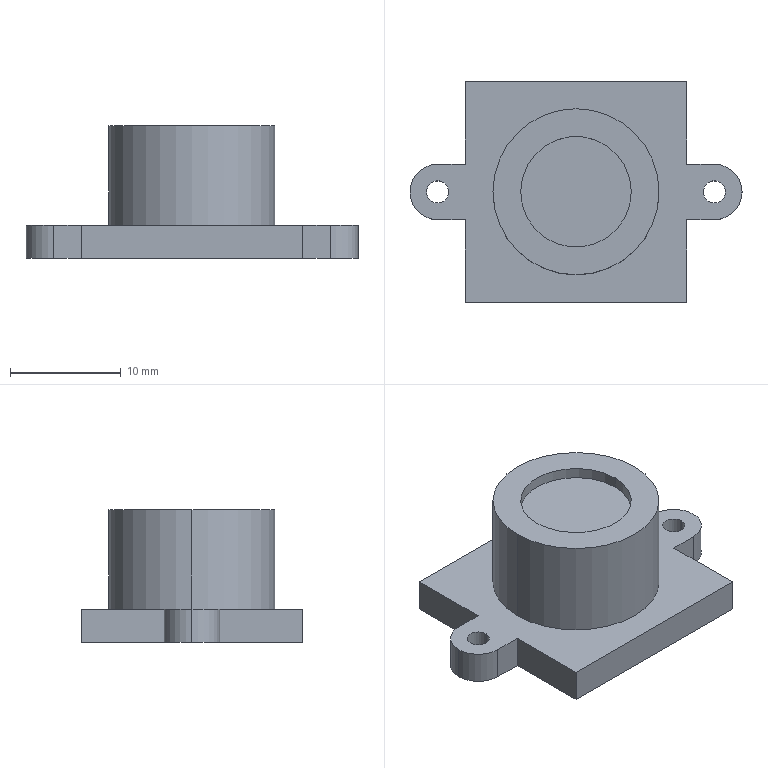Part | SolidWorks | features ICE 4, Extrusion 1, Fillet 1, MirrorPattern 1 | 1 solid | 26 faces | box 30 x 20 x 12 mm | volume 2827 mm3 | plane 14 | cylinder 12 | commonest cylinder face diameters 2 x4 5 x4 10 x2 15 x2
STEP:
#1=CARTESIAN_POINT('',(-5.,0.,11.));
#2=VERTEX_POINT('',#1);
#3=CARTESIAN_POINT('',(5.,0.,11.));
#4=VERTEX_POINT('',#3);
#5=CARTESIAN_POINT('',(0.,0.,11.));
#6=DIRECTION('',(0.,0.,1.));
#7=DIRECTION('',(1.,0.,0.));
#8=AXIS2_PLACEMENT_3D('',#5,#6,#7);
#9=CIRCLE('',#8,5.);
#10=EDGE_CURVE('',#2,#4,#9,.T.);
#11=ORIENTED_EDGE('',*,*,#10,.F.);
#12=CARTESIAN_POINT('',(-5.,0.,12.));
#13=VERTEX_POINT('',#12);
#14=CARTESIAN_POINT('',(-5.,0.,11.));
#15=DIRECTION('',(0.,0.,1.));
#16=VECTOR('',#15,1000.);
#17=LINE('',#14,#16);
#18=EDGE_CURVE('',#2,#13,#17,.T.);
#19=ORIENTED_EDGE('',*,*,#18,.T.);
#20=CARTESIAN_POINT('',(5.,0.,12.));
#21=VERTEX_POINT('',#20);
#22=CARTESIAN_POINT('',(0.,0.,12.));
#23=DIRECTION('',(0.,0.,1.));
#24=DIRECTION('',(1.,0.,0.));
#25=AXIS2_PLACEMENT_3D('',#22,#23,#24);
#26=CIRCLE('',#25,5.);
#27=EDGE_CURVE('',#13,#21,#26,.T.);
#28=ORIENTED_EDGE('',*,*,#27,.T.);
#29=CARTESIAN_POINT('',(5.,0.,11.));
#30=DIRECTION('',(0.,0.,1.));
#31=VECTOR('',#30,1000.);
#32=LINE('',#29,#31);
#33=EDGE_CURVE('',#4,#21,#32,.T.);
#34=ORIENTED_EDGE('',*,*,#33,.F.);
#35=EDGE_LOOP('',(#11,#19,#28,#34));
#36=FACE_OUTER_BOUND('',#35,.T.);
#37=CARTESIAN_POINT('',(0.,0.,11.));
#38=DIRECTION('',(0.,0.,1.));
#39=DIRECTION('',(1.,0.,0.));
#40=AXIS2_PLACEMENT_3D('',#37,#38,#39);
#41=CYLINDRICAL_SURFACE('',#40,5.);
#42=ADVANCED_FACE('',(#36),#41,.F.);
#43=CARTESIAN_POINT('',(7.5,0.,12.));
#44=VERTEX_POINT('',#43);
#45=CARTESIAN_POINT('',(-7.5,0.,12.));
#46=VERTEX_POINT('',#45);
#47=CARTESIAN_POINT('',(0.,0.,12.));
#48=DIRECTION('',(0.,0.,1.));
#49=DIRECTION('',(1.,0.,0.));
#50=AXIS2_PLACEMENT_3D('',#47,#48,#49);
#51=CIRCLE('',#50,7.5);
#52=EDGE_CURVE('',#44,#46,#51,.T.);
#53=ORIENTED_EDGE('',*,*,#52,.F.);
#54=CARTESIAN_POINT('',(7.5,0.,3.));
#55=VERTEX_POINT('',#54);
#56=CARTESIAN_POINT('',(7.5,0.,12.));
#57=DIRECTION('',(0.,0.,-1.));
#58=VECTOR('',#57,1000.);
#59=LINE('',#56,#58);
#60=EDGE_CURVE('',#44,#55,#59,.T.);
#61=ORIENTED_EDGE('',*,*,#60,.T.);
#62=CARTESIAN_POINT('',(-7.5,0.,3.));
#63=VERTEX_POINT('',#62);
#64=CARTESIAN_POINT('',(0.,0.,3.));
#65=DIRECTION('',(0.,0.,1.));
#66=DIRECTION('',(1.,0.,0.));
#67=AXIS2_PLACEMENT_3D('',#64,#65,#66);
#68=CIRCLE('',#67,7.5);
#69=EDGE_CURVE('',#55,#63,#68,.T.);
#70=ORIENTED_EDGE('',*,*,#69,.T.);
#71=CARTESIAN_POINT('',(-7.5,0.,12.));
#72=DIRECTION('',(0.,0.,-1.));
#73=VECTOR('',#72,1000.);
#74=LINE('',#71,#73);
#75=EDGE_CURVE('',#46,#63,#74,.T.);
#76=ORIENTED_EDGE('',*,*,#75,.F.);
#77=EDGE_LOOP('',(#53,#61,#70,#76));
#78=FACE_OUTER_BOUND('',#77,.T.);
#79=CARTESIAN_POINT('',(0.,0.,12.));
#80=DIRECTION('',(0.,0.,-1.));
#81=DIRECTION('',(-1.,0.,0.));
#82=AXIS2_PLACEMENT_3D('',#79,#80,#81);
#83=CYLINDRICAL_SURFACE('',#82,7.5);
#84=ADVANCED_FACE('',(#78),#83,.T.);
#85=CARTESIAN_POINT('',(11.5,0.,0.));
#86=VERTEX_POINT('',#85);
#87=CARTESIAN_POINT('',(13.5,0.,0.));
#88=VERTEX_POINT('',#87);
#89=CARTESIAN_POINT('',(12.5,0.,0.));
#90=DIRECTION('',(0.,0.,1.));
#91=DIRECTION('',(1.,0.,0.));
#92=AXIS2_PLACEMENT_3D('',#89,#90,#91);
#93=CIRCLE('',#92,1.);
#94=EDGE_CURVE('',#86,#88,#93,.T.);
#95=ORIENTED_EDGE('',*,*,#94,.F.);
#96=CARTESIAN_POINT('',(11.5,0.,3.));
#97=VERTEX_POINT('',#96);
#98=CARTESIAN_POINT('',(11.5,0.,-2.828));
#99=DIRECTION('',(0.,0.,1.));
#100=VECTOR('',#99,1000.);
#101=LINE('',#98,#100);
#102=EDGE_CURVE('',#86,#97,#101,.T.);
#103=ORIENTED_EDGE('',*,*,#102,.T.);
#104=CARTESIAN_POINT('',(13.5,0.,3.));
#105=VERTEX_POINT('',#104);
#106=CARTESIAN_POINT('',(12.5,0.,3.));
#107=DIRECTION('',(0.,0.,-1.));
#108=DIRECTION('',(-1.,0.,0.));
#109=AXIS2_PLACEMENT_3D('',#106,#107,#108);
#110=CIRCLE('',#109,1.);
#111=EDGE_CURVE('',#105,#97,#110,.T.);
#112=ORIENTED_EDGE('',*,*,#111,.F.);
#113=CARTESIAN_POINT('',(13.5,0.,-2.828));
#114=DIRECTION('',(0.,0.,1.));
#115=VECTOR('',#114,1000.);
#116=LINE('',#113,#115);
#117=EDGE_CURVE('',#88,#105,#116,.T.);
#118=ORIENTED_EDGE('',*,*,#117,.F.);
#119=EDGE_LOOP('',(#95,#103,#112,#118));
#120=FACE_OUTER_BOUND('',#119,.T.);
#121=CARTESIAN_POINT('',(12.5,0.,-2.828));
#122=DIRECTION('',(0.,0.,1.));
#123=DIRECTION('',(1.,0.,0.));
#124=AXIS2_PLACEMENT_3D('',#121,#122,#123);
#125=CYLINDRICAL_SURFACE('',#124,1.);
#126=ADVANCED_FACE('',(#120),#125,.F.);
#127=CARTESIAN_POINT('',(-11.5,0.,0.));
#128=VERTEX_POINT('',#127);
#129=CARTESIAN_POINT('',(-13.5,0.,0.));
#130=VERTEX_POINT('',#129);
#131=CARTESIAN_POINT('',(-12.5,0.,0.));
#132=DIRECTION('',(0.,0.,-1.));
#133=DIRECTION('',(1.,0.,0.));
#134=AXIS2_PLACEMENT_3D('',#131,#132,#133);
#135=CIRCLE('',#134,1.);
#136=EDGE_CURVE('',#128,#130,#135,.T.);
#137=ORIENTED_EDGE('',*,*,#136,.T.);
#138=CARTESIAN_POINT('',(-13.5,0.,3.));
#139=VERTEX_POINT('',#138);
#140=CARTESIAN_POINT('',(-13.5,0.,-2.828));
#141=DIRECTION('',(0.,0.,1.));
#142=VECTOR('',#141,1000.);
#143=LINE('',#140,#142);
#144=EDGE_CURVE('',#130,#139,#143,.T.);
#145=ORIENTED_EDGE('',*,*,#144,.T.);
#146=CARTESIAN_POINT('',(-11.5,0.,3.));
#147=VERTEX_POINT('',#146);
#148=CARTESIAN_POINT('',(-12.5,0.,3.));
#149=DIRECTION('',(0.,0.,1.));
#150=DIRECTION('',(1.,0.,0.));
#151=AXIS2_PLACEMENT_3D('',#148,#149,#150);
#152=CIRCLE('',#151,1.);
#153=EDGE_CURVE('',#139,#147,#152,.T.);
#154=ORIENTED_EDGE('',*,*,#153,.T.);
#155=CARTESIAN_POINT('',(-11.5,0.,-2.828));
#156=DIRECTION('',(0.,0.,1.));
#157=VECTOR('',#156,1000.);
#158=LINE('',#155,#157);
#159=EDGE_CURVE('',#128,#147,#158,.T.);
#160=ORIENTED_EDGE('',*,*,#159,.F.);
#161=EDGE_LOOP('',(#137,#145,#154,#160));
#162=FACE_OUTER_BOUND('',#161,.T.);
#163=CARTESIAN_POINT('',(-12.5,0.,-2.828));
#164=DIRECTION('',(0.,0.,1.));
#165=DIRECTION('',(1.,0.,0.));
#166=AXIS2_PLACEMENT_3D('',#163,#164,#165);
#167=CYLINDRICAL_SURFACE('',#166,1.);
#168=ADVANCED_FACE('',(#162),#167,.F.);
#169=CARTESIAN_POINT('',(10.,2.5,0.));
#170=VERTEX_POINT('',#169);
#171=CARTESIAN_POINT('',(10.,2.5,3.));
#172=VERTEX_POINT('',#171);
#173=CARTESIAN_POINT('',(10.,2.5,-7.071));
#174=DIRECTION('',(0.,0.,1.));
#175=VECTOR('',#174,1000.);
#176=LINE('',#173,#175);
#177=EDGE_CURVE('',#170,#172,#176,.T.);
#178=ORIENTED_EDGE('',*,*,#177,.F.);
#179=CARTESIAN_POINT('',(10.,10.,0.));
#180=VERTEX_POINT('',#179);
#181=CARTESIAN_POINT('',(10.,10.,0.));
#182=DIRECTION('',(0.,1.,0.));
#183=VECTOR('',#182,1000.);
#184=LINE('',#181,#183);
#185=EDGE_CURVE('',#170,#180,#184,.T.);
#186=ORIENTED_EDGE('',*,*,#185,.T.);
#187=CARTESIAN_POINT('',(10.,10.,3.));
#188=VERTEX_POINT('',#187);
#189=CARTESIAN_POINT('',(10.,10.,3.));
#190=DIRECTION('',(0.,0.,-1.));
#191=VECTOR('',#190,1000.);
#192=LINE('',#189,#191);
#193=EDGE_CURVE('',#188,#180,#192,.T.);
#194=ORIENTED_EDGE('',*,*,#193,.F.);
#195=CARTESIAN_POINT('',(10.,10.,3.));
#196=DIRECTION('',(0.,1.,0.));
#197=VECTOR('',#196,1000.);
#198=LINE('',#195,#197);
#199=EDGE_CURVE('',#172,#188,#198,.T.);
#200=ORIENTED_EDGE('',*,*,#199,.F.);
#201=EDGE_LOOP('',(#178,#186,#194,#200));
#202=FACE_OUTER_BOUND('',#201,.T.);
#203=CARTESIAN_POINT('',(10.,10.,3.));
#204=DIRECTION('',(-1.,0.,0.));
#205=DIRECTION('',(0.,-1.,0.));
#206=AXIS2_PLACEMENT_3D('',#203,#204,#205);
#207=PLANE('',#206);
#208=ADVANCED_FACE('',(#202),#207,.F.);
#209=CARTESIAN_POINT('',(-10.,-2.5,0.));
#210=VERTEX_POINT('',#209);
#211=CARTESIAN_POINT('',(-10.,-2.5,3.));
#212=VERTEX_POINT('',#211);
#213=CARTESIAN_POINT('',(-10.,-2.5,-7.071));
#214=DIRECTION('',(0.,0.,1.));
#215=VECTOR('',#214,1000.);
#216=LINE('',#213,#215);
#217=EDGE_CURVE('',#210,#212,#216,.T.);
#218=ORIENTED_EDGE('',*,*,#217,.F.);
#219=CARTESIAN_POINT('',(-10.,-10.,0.));
#220=VERTEX_POINT('',#219);
#221=CARTESIAN_POINT('',(-10.,10.,0.));
#222=DIRECTION('',(0.,-1.,0.));
#223=VECTOR('',#222,1000.);
#224=LINE('',#221,#223);
#225=EDGE_CURVE('',#210,#220,#224,.T.);
#226=ORIENTED_EDGE('',*,*,#225,.T.);
#227=CARTESIAN_POINT('',(-10.,-10.,3.));
#228=VERTEX_POINT('',#227);
#229=CARTESIAN_POINT('',(-10.,-10.,3.));
#230=DIRECTION('',(0.,0.,-1.));
#231=VECTOR('',#230,1000.);
#232=LINE('',#229,#231);
#233=EDGE_CURVE('',#228,#220,#232,.T.);
#234=ORIENTED_EDGE('',*,*,#233,.F.);
#235=CARTESIAN_POINT('',(-10.,10.,3.));
#236=DIRECTION('',(0.,-1.,0.));
#237=VECTOR('',#236,1000.);
#238=LINE('',#235,#237);
#239=EDGE_CURVE('',#212,#228,#238,.T.);
#240=ORIENTED_EDGE('',*,*,#239,.F.);
#241=EDGE_LOOP('',(#218,#226,#234,#240));
#242=FACE_OUTER_BOUND('',#241,.T.);
#243=CARTESIAN_POINT('',(-10.,10.,3.));
#244=DIRECTION('',(1.,0.,0.));
#245=DIRECTION('',(0.,1.,0.));
#246=AXIS2_PLACEMENT_3D('',#243,#244,#245);
#247=PLANE('',#246);
#248=ADVANCED_FACE('',(#242),#247,.F.);
#249=CARTESIAN_POINT('',(10.,-10.,0.));
#250=VERTEX_POINT('',#249);
#251=CARTESIAN_POINT('',(10.,-2.5,0.));
#252=VERTEX_POINT('',#251);
#253=CARTESIAN_POINT('',(10.,10.,0.));
#254=DIRECTION('',(0.,1.,0.));
#255=VECTOR('',#254,1000.);
#256=LINE('',#253,#255);
#257=EDGE_CURVE('',#250,#252,#256,.T.);
#258=ORIENTED_EDGE('',*,*,#257,.T.);
#259=CARTESIAN_POINT('',(10.,-2.5,3.));
#260=VERTEX_POINT('',#259);
#261=CARTESIAN_POINT('',(10.,-2.5,-7.071));
#262=DIRECTION('',(0.,0.,1.));
#263=VECTOR('',#262,1000.);
#264=LINE('',#261,#263);
#265=EDGE_CURVE('',#252,#260,#264,.T.);
#266=ORIENTED_EDGE('',*,*,#265,.T.);
#267=CARTESIAN_POINT('',(10.,-10.,3.));
#268=VERTEX_POINT('',#267);
#269=CARTESIAN_POINT('',(10.,10.,3.));
#270=DIRECTION('',(0.,1.,0.));
#271=VECTOR('',#270,1000.);
#272=LINE('',#269,#271);
#273=EDGE_CURVE('',#268,#260,#272,.T.);
#274=ORIENTED_EDGE('',*,*,#273,.F.);
#275=CARTESIAN_POINT('',(10.,-10.,3.));
#276=DIRECTION('',(0.,0.,-1.));
#277=VECTOR('',#276,1000.);
#278=LINE('',#275,#277);
#279=EDGE_CURVE('',#268,#250,#278,.T.);
#280=ORIENTED_EDGE('',*,*,#279,.T.);
#281=EDGE_LOOP('',(#258,#266,#274,#280));
#282=FACE_OUTER_BOUND('',#281,.T.);
#283=CARTESIAN_POINT('',(10.,10.,3.));
#284=DIRECTION('',(-1.,0.,0.));
#285=DIRECTION('',(0.,-1.,0.));
#286=AXIS2_PLACEMENT_3D('',#283,#284,#285);
#287=PLANE('',#286);
#288=ADVANCED_FACE('',(#282),#287,.F.);
#289=CARTESIAN_POINT('',(-10.,10.,0.));
#290=VERTEX_POINT('',#289);
#291=CARTESIAN_POINT('',(-10.,10.,0.));
#292=DIRECTION('',(-1.,0.,0.));
#293=VECTOR('',#292,1000.);
#294=LINE('',#291,#293);
#295=EDGE_CURVE('',#180,#290,#294,.T.);
#296=ORIENTED_EDGE('',*,*,#295,.T.);
#297=CARTESIAN_POINT('',(-10.,10.,3.));
#298=VERTEX_POINT('',#297);
#299=CARTESIAN_POINT('',(-10.,10.,3.));
#300=DIRECTION('',(0.,0.,-1.));
#301=VECTOR('',#300,1000.);
#302=LINE('',#299,#301);
#303=EDGE_CURVE('',#298,#290,#302,.T.);
#304=ORIENTED_EDGE('',*,*,#303,.F.);
#305=CARTESIAN_POINT('',(-10.,10.,3.));
#306=DIRECTION('',(-1.,0.,0.));
#307=VECTOR('',#306,1000.);
#308=LINE('',#305,#307);
#309=EDGE_CURVE('',#188,#298,#308,.T.);
#310=ORIENTED_EDGE('',*,*,#309,.F.);
#311=ORIENTED_EDGE('',*,*,#193,.T.);
#312=EDGE_LOOP('',(#296,#304,#310,#311));
#313=FACE_OUTER_BOUND('',#312,.T.);
#314=CARTESIAN_POINT('',(-10.,10.,3.));
#315=DIRECTION('',(0.,-1.,0.));
#316=DIRECTION('',(0.,0.,-1.));
#317=AXIS2_PLACEMENT_3D('',#314,#315,#316);
#318=PLANE('',#317);
#319=ADVANCED_FACE('',(#313),#318,.F.);
#320=CARTESIAN_POINT('',(-10.,2.5,0.));
#321=VERTEX_POINT('',#320);
#322=CARTESIAN_POINT('',(-10.,10.,0.));
#323=DIRECTION('',(0.,-1.,0.));
#324=VECTOR('',#323,1000.);
#325=LINE('',#322,#324);
#326=EDGE_CURVE('',#290,#321,#325,.T.);
#327=ORIENTED_EDGE('',*,*,#326,.T.);
#328=CARTESIAN_POINT('',(-10.,2.5,3.));
#329=VERTEX_POINT('',#328);
#330=CARTESIAN_POINT('',(-10.,2.5,-7.071));
#331=DIRECTION('',(0.,0.,1.));
#332=VECTOR('',#331,1000.);
#333=LINE('',#330,#332);
#334=EDGE_CURVE('',#321,#329,#333,.T.);
#335=ORIENTED_EDGE('',*,*,#334,.T.);
#336=CARTESIAN_POINT('',(-10.,10.,3.));
#337=DIRECTION('',(0.,-1.,0.));
#338=VECTOR('',#337,1000.);
#339=LINE('',#336,#338);
#340=EDGE_CURVE('',#298,#329,#339,.T.);
#341=ORIENTED_EDGE('',*,*,#340,.F.);
#342=ORIENTED_EDGE('',*,*,#303,.T.);
#343=EDGE_LOOP('',(#327,#335,#341,#342));
#344=FACE_OUTER_BOUND('',#343,.T.);
#345=CARTESIAN_POINT('',(-10.,10.,3.));
#346=DIRECTION('',(1.,0.,0.));
#347=DIRECTION('',(0.,1.,0.));
#348=AXIS2_PLACEMENT_3D('',#345,#346,#347);
#349=PLANE('',#348);
#350=ADVANCED_FACE('',(#344),#349,.F.);
#351=CARTESIAN_POINT('',(-10.,-10.,0.));
#352=DIRECTION('',(1.,0.,0.));
#353=VECTOR('',#352,1000.);
#354=LINE('',#351,#353);
#355=EDGE_CURVE('',#220,#250,#354,.T.);
#356=ORIENTED_EDGE('',*,*,#355,.T.);
#357=ORIENTED_EDGE('',*,*,#279,.F.);
#358=CARTESIAN_POINT('',(-10.,-10.,3.));
#359=DIRECTION('',(1.,0.,0.));
#360=VECTOR('',#359,1000.);
#361=LINE('',#358,#360);
#362=EDGE_CURVE('',#228,#268,#361,.T.);
#363=ORIENTED_EDGE('',*,*,#362,.F.);
#364=ORIENTED_EDGE('',*,*,#233,.T.);
#365=EDGE_LOOP('',(#356,#357,#363,#364));
#366=FACE_OUTER_BOUND('',#365,.T.);
#367=CARTESIAN_POINT('',(-10.,-10.,3.));
#368=DIRECTION('',(0.,1.,0.));
#369=DIRECTION('',(0.,0.,1.));
#370=AXIS2_PLACEMENT_3D('',#367,#368,#369);
#371=PLANE('',#370);
#372=ADVANCED_FACE('',(#366),#371,.F.);
#373=CARTESIAN_POINT('',(0.,0.,3.));
#374=DIRECTION('',(0.,0.,1.));
#375=DIRECTION('',(1.,0.,0.));
#376=AXIS2_PLACEMENT_3D('',#373,#374,#375);
#377=CIRCLE('',#376,7.5);
#378=EDGE_CURVE('',#63,#55,#377,.T.);
#379=ORIENTED_EDGE('',*,*,#378,.F.);
#380=ORIENTED_EDGE('',*,*,#69,.F.);
#381=EDGE_LOOP('',(#379,#380));
#382=FACE_BOUND('',#381,.T.);
#383=ORIENTED_EDGE('',*,*,#111,.T.);
#384=CARTESIAN_POINT('',(12.5,0.,3.));
#385=DIRECTION('',(0.,0.,-1.));
#386=DIRECTION('',(-1.,0.,0.));
#387=AXIS2_PLACEMENT_3D('',#384,#385,#386);
#388=CIRCLE('',#387,1.);
#389=EDGE_CURVE('',#97,#105,#388,.T.);
#390=ORIENTED_EDGE('',*,*,#389,.T.);
#391=EDGE_LOOP('',(#383,#390));
#392=FACE_BOUND('',#391,.T.);
#393=CARTESIAN_POINT('',(-12.5,0.,3.));
#394=DIRECTION('',(0.,0.,1.));
#395=DIRECTION('',(1.,0.,0.));
#396=AXIS2_PLACEMENT_3D('',#393,#394,#395);
#397=CIRCLE('',#396,1.);
#398=EDGE_CURVE('',#147,#139,#397,.T.);
#399=ORIENTED_EDGE('',*,*,#398,.F.);
#400=ORIENTED_EDGE('',*,*,#153,.F.);
#401=EDGE_LOOP('',(#399,#400));
#402=FACE_BOUND('',#401,.T.);
#403=CARTESIAN_POINT('',(12.5,-2.5,3.));
#404=VERTEX_POINT('',#403);
#405=CARTESIAN_POINT('',(15.,0.,3.));
#406=VERTEX_POINT('',#405);
#407=CARTESIAN_POINT('',(12.5,0.,3.));
#408=DIRECTION('',(0.,0.,1.));
#409=DIRECTION('',(1.,0.,0.));
#410=AXIS2_PLACEMENT_3D('',#407,#408,#409);
#411=CIRCLE('',#410,2.5);
#412=EDGE_CURVE('',#404,#406,#411,.T.);
#413=ORIENTED_EDGE('',*,*,#412,.T.);
#414=CARTESIAN_POINT('',(12.5,2.5,3.));
#415=VERTEX_POINT('',#414);
#416=CARTESIAN_POINT('',(12.5,0.,3.));
#417=DIRECTION('',(0.,0.,1.));
#418=DIRECTION('',(1.,0.,0.));
#419=AXIS2_PLACEMENT_3D('',#416,#417,#418);
#420=CIRCLE('',#419,2.5);
#421=EDGE_CURVE('',#406,#415,#420,.T.);
#422=ORIENTED_EDGE('',*,*,#421,.T.);
#423=CARTESIAN_POINT('',(10.,2.5,3.));
#424=DIRECTION('',(1.,0.,0.));
#425=VECTOR('',#424,1000.);
#426=LINE('',#423,#425);
#427=EDGE_CURVE('',#172,#415,#426,.T.);
#428=ORIENTED_EDGE('',*,*,#427,.F.);
#429=ORIENTED_EDGE('',*,*,#199,.T.);
#430=ORIENTED_EDGE('',*,*,#309,.T.);
#431=ORIENTED_EDGE('',*,*,#340,.T.);
#432=CARTESIAN_POINT('',(-12.5,2.5,3.));
#433=VERTEX_POINT('',#432);
#434=CARTESIAN_POINT('',(-10.,2.5,3.));
#435=DIRECTION('',(-1.,0.,0.));
#436=VECTOR('',#435,1000.);
#437=LINE('',#434,#436);
#438=EDGE_CURVE('',#329,#433,#437,.T.);
#439=ORIENTED_EDGE('',*,*,#438,.T.);
#440=CARTESIAN_POINT('',(-15.,0.,3.));
#441=VERTEX_POINT('',#440);
#442=CARTESIAN_POINT('',(-12.5,0.,3.));
#443=DIRECTION('',(0.,0.,1.));
#444=DIRECTION('',(1.,0.,0.));
#445=AXIS2_PLACEMENT_3D('',#442,#443,#444);
#446=CIRCLE('',#445,2.5);
#447=EDGE_CURVE('',#433,#441,#446,.T.);
#448=ORIENTED_EDGE('',*,*,#447,.T.);
#449=CARTESIAN_POINT('',(-12.5,-2.5,3.));
#450=VERTEX_POINT('',#449);
#451=CARTESIAN_POINT('',(-12.5,0.,3.));
#452=DIRECTION('',(0.,0.,1.));
#453=DIRECTION('',(1.,0.,0.));
#454=AXIS2_PLACEMENT_3D('',#451,#452,#453);
#455=CIRCLE('',#454,2.5);
#456=EDGE_CURVE('',#441,#450,#455,.T.);
#457=ORIENTED_EDGE('',*,*,#456,.T.);
#458=CARTESIAN_POINT('',(-15.,-2.5,3.));
#459=DIRECTION('',(1.,0.,0.));
#460=VECTOR('',#459,1000.);
#461=LINE('',#458,#460);
#462=EDGE_CURVE('',#450,#212,#461,.T.);
#463=ORIENTED_EDGE('',*,*,#462,.T.);
#464=ORIENTED_EDGE('',*,*,#239,.T.);
#465=ORIENTED_EDGE('',*,*,#362,.T.);
#466=ORIENTED_EDGE('',*,*,#273,.T.);
#467=CARTESIAN_POINT('',(15.,-2.5,3.));
#468=DIRECTION('',(-1.,0.,0.));
#469=VECTOR('',#468,1000.);
#470=LINE('',#467,#469);
#471=EDGE_CURVE('',#404,#260,#470,.T.);
#472=ORIENTED_EDGE('',*,*,#471,.F.);
#473=EDGE_LOOP('',(#413,#422,#428,#429,#430,#431,#439,#448,#457,#463,#464,#465,#466,#472));
#474=FACE_OUTER_BOUND('',#473,.T.);
#475=CARTESIAN_POINT('',(0.,0.,3.));
#476=DIRECTION('',(0.,0.,1.));
#477=DIRECTION('',(1.,0.,0.));
#478=AXIS2_PLACEMENT_3D('',#475,#476,#477);
#479=PLANE('',#478);
#480=ADVANCED_FACE('',(#382,#392,#402,#474),#479,.T.);
#481=CARTESIAN_POINT('',(12.5,0.,0.));
#482=DIRECTION('',(0.,0.,1.));
#483=DIRECTION('',(1.,0.,0.));
#484=AXIS2_PLACEMENT_3D('',#481,#482,#483);
#485=CIRCLE('',#484,1.);
#486=EDGE_CURVE('',#88,#86,#485,.T.);
#487=ORIENTED_EDGE('',*,*,#486,.T.);
#488=ORIENTED_EDGE('',*,*,#94,.T.);
#489=EDGE_LOOP('',(#487,#488));
#490=FACE_BOUND('',#489,.T.);
#491=ORIENTED_EDGE('',*,*,#136,.F.);
#492=CARTESIAN_POINT('',(-12.5,0.,0.));
#493=DIRECTION('',(0.,0.,-1.));
#494=DIRECTION('',(1.,0.,0.));
#495=AXIS2_PLACEMENT_3D('',#492,#493,#494);
#496=CIRCLE('',#495,1.);
#497=EDGE_CURVE('',#130,#128,#496,.T.);
#498=ORIENTED_EDGE('',*,*,#497,.F.);
#499=EDGE_LOOP('',(#491,#498));
#500=FACE_BOUND('',#499,.T.);
#501=CARTESIAN_POINT('',(12.5,2.5,0.));
#502=VERTEX_POINT('',#501);
#503=CARTESIAN_POINT('',(10.,2.5,0.));
#504=DIRECTION('',(-1.,0.,0.));
#505=VECTOR('',#504,1000.);
#506=LINE('',#503,#505);
#507=EDGE_CURVE('',#502,#170,#506,.T.);
#508=ORIENTED_EDGE('',*,*,#507,.F.);
#509=CARTESIAN_POINT('',(15.,0.,0.));
#510=VERTEX_POINT('',#509);
#511=CARTESIAN_POINT('',(12.5,0.,0.));
#512=DIRECTION('',(0.,0.,-1.));
#513=DIRECTION('',(1.,0.,0.));
#514=AXIS2_PLACEMENT_3D('',#511,#512,#513);
#515=CIRCLE('',#514,2.5);
#516=EDGE_CURVE('',#502,#510,#515,.T.);
#517=ORIENTED_EDGE('',*,*,#516,.T.);
#518=CARTESIAN_POINT('',(12.5,-2.5,0.));
#519=VERTEX_POINT('',#518);
#520=CARTESIAN_POINT('',(12.5,0.,0.));
#521=DIRECTION('',(0.,0.,-1.));
#522=DIRECTION('',(1.,0.,0.));
#523=AXIS2_PLACEMENT_3D('',#520,#521,#522);
#524=CIRCLE('',#523,2.5);
#525=EDGE_CURVE('',#510,#519,#524,.T.);
#526=ORIENTED_EDGE('',*,*,#525,.T.);
#527=CARTESIAN_POINT('',(15.,-2.5,0.));
#528=DIRECTION('',(1.,0.,0.));
#529=VECTOR('',#528,1000.);
#530=LINE('',#527,#529);
#531=EDGE_CURVE('',#252,#519,#530,.T.);
#532=ORIENTED_EDGE('',*,*,#531,.F.);
#533=ORIENTED_EDGE('',*,*,#257,.F.);
#534=ORIENTED_EDGE('',*,*,#355,.F.);
#535=ORIENTED_EDGE('',*,*,#225,.F.);
#536=CARTESIAN_POINT('',(-12.5,-2.5,0.));
#537=VERTEX_POINT('',#536);
#538=CARTESIAN_POINT('',(-15.,-2.5,0.));
#539=DIRECTION('',(-1.,0.,0.));
#540=VECTOR('',#539,1000.);
#541=LINE('',#538,#540);
#542=EDGE_CURVE('',#210,#537,#541,.T.);
#543=ORIENTED_EDGE('',*,*,#542,.T.);
#544=CARTESIAN_POINT('',(-15.,0.,0.));
#545=VERTEX_POINT('',#544);
#546=CARTESIAN_POINT('',(-12.5,0.,0.));
#547=DIRECTION('',(0.,0.,-1.));
#548=DIRECTION('',(1.,0.,0.));
#549=AXIS2_PLACEMENT_3D('',#546,#547,#548);
#550=CIRCLE('',#549,2.5);
#551=EDGE_CURVE('',#537,#545,#550,.T.);
#552=ORIENTED_EDGE('',*,*,#551,.T.);
#553=CARTESIAN_POINT('',(-12.5,2.5,0.));
#554=VERTEX_POINT('',#553);
#555=CARTESIAN_POINT('',(-12.5,0.,0.));
#556=DIRECTION('',(0.,0.,-1.));
#557=DIRECTION('',(1.,0.,0.));
#558=AXIS2_PLACEMENT_3D('',#555,#556,#557);
#559=CIRCLE('',#558,2.5);
#560=EDGE_CURVE('',#545,#554,#559,.T.);
#561=ORIENTED_EDGE('',*,*,#560,.T.);
#562=CARTESIAN_POINT('',(-10.,2.5,0.));
#563=DIRECTION('',(1.,0.,0.));
#564=VECTOR('',#563,1000.);
#565=LINE('',#562,#564);
#566=EDGE_CURVE('',#554,#321,#565,.T.);
#567=ORIENTED_EDGE('',*,*,#566,.T.);
#568=ORIENTED_EDGE('',*,*,#326,.F.);
#569=ORIENTED_EDGE('',*,*,#295,.F.);
#570=ORIENTED_EDGE('',*,*,#185,.F.);
#571=EDGE_LOOP('',(#508,#517,#526,#532,#533,#534,#535,#543,#552,#561,#567,#568,#569,#570));
#572=FACE_OUTER_BOUND('',#571,.T.);
#573=CARTESIAN_POINT('',(0.,0.,0.));
#574=DIRECTION('',(0.,0.,1.));
#575=DIRECTION('',(1.,0.,0.));
#576=AXIS2_PLACEMENT_3D('',#573,#574,#575);
#577=PLANE('',#576);
#578=ADVANCED_FACE('',(#490,#500,#572),#577,.F.);
#579=ORIENTED_EDGE('',*,*,#462,.F.);
#580=CARTESIAN_POINT('',(-12.5,-2.5,-7.071));
#581=DIRECTION('',(0.,0.,-1.));
#582=VECTOR('',#581,1000.);
#583=LINE('',#580,#582);
#584=EDGE_CURVE('',#450,#537,#583,.T.);
#585=ORIENTED_EDGE('',*,*,#584,.T.);
#586=ORIENTED_EDGE('',*,*,#542,.F.);
#587=ORIENTED_EDGE('',*,*,#217,.T.);
#588=EDGE_LOOP('',(#579,#585,#586,#587));
#589=FACE_OUTER_BOUND('',#588,.T.);
#590=CARTESIAN_POINT('',(-15.,-2.5,-7.071));
#591=DIRECTION('',(0.,-1.,0.));
#592=DIRECTION('',(1.,0.,0.));
#593=AXIS2_PLACEMENT_3D('',#590,#591,#592);
#594=PLANE('',#593);
#595=ADVANCED_FACE('',(#589),#594,.T.);
#596=ORIENTED_EDGE('',*,*,#566,.F.);
#597=CARTESIAN_POINT('',(-12.5,2.5,-7.071));
#598=DIRECTION('',(0.,0.,1.));
#599=VECTOR('',#598,1000.);
#600=LINE('',#597,#599);
#601=EDGE_CURVE('',#554,#433,#600,.T.);
#602=ORIENTED_EDGE('',*,*,#601,.T.);
#603=ORIENTED_EDGE('',*,*,#438,.F.);
#604=ORIENTED_EDGE('',*,*,#334,.F.);
#605=EDGE_LOOP('',(#596,#602,#603,#604));
#606=FACE_OUTER_BOUND('',#605,.T.);
#607=CARTESIAN_POINT('',(-10.,2.5,-7.071));
#608=DIRECTION('',(0.,1.,0.));
#609=DIRECTION('',(-1.,0.,0.));
#610=AXIS2_PLACEMENT_3D('',#607,#608,#609);
#611=PLANE('',#610);
#612=ADVANCED_FACE('',(#606),#611,.T.);
#613=ORIENTED_EDGE('',*,*,#144,.F.);
#614=ORIENTED_EDGE('',*,*,#497,.T.);
#615=ORIENTED_EDGE('',*,*,#159,.T.);
#616=ORIENTED_EDGE('',*,*,#398,.T.);
#617=EDGE_LOOP('',(#613,#614,#615,#616));
#618=FACE_OUTER_BOUND('',#617,.T.);
#619=CARTESIAN_POINT('',(-12.5,0.,-2.828));
#620=DIRECTION('',(0.,0.,1.));
#621=DIRECTION('',(1.,0.,0.));
#622=AXIS2_PLACEMENT_3D('',#619,#620,#621);
#623=CYLINDRICAL_SURFACE('',#622,1.);
#624=ADVANCED_FACE('',(#618),#623,.F.);
#625=CARTESIAN_POINT('',(-15.,0.,-7.071));
#626=DIRECTION('',(0.,0.,1.));
#627=VECTOR('',#626,1000.);
#628=LINE('',#625,#627);
#629=EDGE_CURVE('',#545,#441,#628,.T.);
#630=ORIENTED_EDGE('',*,*,#629,.F.);
#631=ORIENTED_EDGE('',*,*,#551,.F.);
#632=ORIENTED_EDGE('',*,*,#584,.F.);
#633=ORIENTED_EDGE('',*,*,#456,.F.);
#634=EDGE_LOOP('',(#630,#631,#632,#633));
#635=FACE_OUTER_BOUND('',#634,.T.);
#636=CARTESIAN_POINT('',(-12.5,0.,-7.071));
#637=DIRECTION('',(0.,0.,1.));
#638=DIRECTION('',(1.,0.,0.));
#639=AXIS2_PLACEMENT_3D('',#636,#637,#638);
#640=CYLINDRICAL_SURFACE('',#639,2.5);
#641=ADVANCED_FACE('',(#635),#640,.T.);
#642=ORIENTED_EDGE('',*,*,#560,.F.);
#643=ORIENTED_EDGE('',*,*,#629,.T.);
#644=ORIENTED_EDGE('',*,*,#447,.F.);
#645=ORIENTED_EDGE('',*,*,#601,.F.);
#646=EDGE_LOOP('',(#642,#643,#644,#645));
#647=FACE_OUTER_BOUND('',#646,.T.);
#648=CARTESIAN_POINT('',(-12.5,0.,-7.071));
#649=DIRECTION('',(0.,0.,1.));
#650=DIRECTION('',(1.,0.,0.));
#651=AXIS2_PLACEMENT_3D('',#648,#649,#650);
#652=CYLINDRICAL_SURFACE('',#651,2.5);
#653=ADVANCED_FACE('',(#647),#652,.T.);
#654=ORIENTED_EDGE('',*,*,#531,.T.);
#655=CARTESIAN_POINT('',(12.5,-2.5,-7.071));
#656=DIRECTION('',(0.,0.,1.));
#657=VECTOR('',#656,1000.);
#658=LINE('',#655,#657);
#659=EDGE_CURVE('',#519,#404,#658,.T.);
#660=ORIENTED_EDGE('',*,*,#659,.T.);
#661=ORIENTED_EDGE('',*,*,#471,.T.);
#662=ORIENTED_EDGE('',*,*,#265,.F.);
#663=EDGE_LOOP('',(#654,#660,#661,#662));
#664=FACE_OUTER_BOUND('',#663,.T.);
#665=CARTESIAN_POINT('',(15.,-2.5,-7.071));
#666=DIRECTION('',(0.,1.,0.));
#667=DIRECTION('',(-1.,0.,0.));
#668=AXIS2_PLACEMENT_3D('',#665,#666,#667);
#669=PLANE('',#668);
#670=ADVANCED_FACE('',(#664),#669,.F.);
#671=ORIENTED_EDGE('',*,*,#427,.T.);
#672=CARTESIAN_POINT('',(12.5,2.5,-7.071));
#673=DIRECTION('',(0.,0.,-1.));
#674=VECTOR('',#673,1000.);
#675=LINE('',#672,#674);
#676=EDGE_CURVE('',#415,#502,#675,.T.);
#677=ORIENTED_EDGE('',*,*,#676,.T.);
#678=ORIENTED_EDGE('',*,*,#507,.T.);
#679=ORIENTED_EDGE('',*,*,#177,.T.);
#680=EDGE_LOOP('',(#671,#677,#678,#679));
#681=FACE_OUTER_BOUND('',#680,.T.);
#682=CARTESIAN_POINT('',(10.,2.5,-7.071));
#683=DIRECTION('',(0.,-1.,0.));
#684=DIRECTION('',(1.,0.,0.));
#685=AXIS2_PLACEMENT_3D('',#682,#683,#684);
#686=PLANE('',#685);
#687=ADVANCED_FACE('',(#681),#686,.F.);
#688=ORIENTED_EDGE('',*,*,#102,.F.);
#689=ORIENTED_EDGE('',*,*,#486,.F.);
#690=ORIENTED_EDGE('',*,*,#117,.T.);
#691=ORIENTED_EDGE('',*,*,#389,.F.);
#692=EDGE_LOOP('',(#688,#689,#690,#691));
#693=FACE_OUTER_BOUND('',#692,.T.);
#694=CARTESIAN_POINT('',(12.5,0.,-2.828));
#695=DIRECTION('',(0.,0.,1.));
#696=DIRECTION('',(1.,0.,0.));
#697=AXIS2_PLACEMENT_3D('',#694,#695,#696);
#698=CYLINDRICAL_SURFACE('',#697,1.);
#699=ADVANCED_FACE('',(#693),#698,.F.);
#700=ORIENTED_EDGE('',*,*,#659,.F.);
#701=ORIENTED_EDGE('',*,*,#525,.F.);
#702=CARTESIAN_POINT('',(15.,0.,-7.071));
#703=DIRECTION('',(0.,0.,-1.));
#704=VECTOR('',#703,1000.);
#705=LINE('',#702,#704);
#706=EDGE_CURVE('',#406,#510,#705,.T.);
#707=ORIENTED_EDGE('',*,*,#706,.F.);
#708=ORIENTED_EDGE('',*,*,#412,.F.);
#709=EDGE_LOOP('',(#700,#701,#707,#708));
#710=FACE_OUTER_BOUND('',#709,.T.);
#711=CARTESIAN_POINT('',(12.5,0.,-7.071));
#712=DIRECTION('',(0.,0.,1.));
#713=DIRECTION('',(1.,0.,0.));
#714=AXIS2_PLACEMENT_3D('',#711,#712,#713);
#715=CYLINDRICAL_SURFACE('',#714,2.5);
#716=ADVANCED_FACE('',(#710),#715,.T.);
#717=ORIENTED_EDGE('',*,*,#516,.F.);
#718=ORIENTED_EDGE('',*,*,#676,.F.);
#719=ORIENTED_EDGE('',*,*,#421,.F.);
#720=ORIENTED_EDGE('',*,*,#706,.T.);
#721=EDGE_LOOP('',(#717,#718,#719,#720));
#722=FACE_OUTER_BOUND('',#721,.T.);
#723=CARTESIAN_POINT('',(12.5,0.,-7.071));
#724=DIRECTION('',(0.,0.,1.));
#725=DIRECTION('',(1.,0.,0.));
#726=AXIS2_PLACEMENT_3D('',#723,#724,#725);
#727=CYLINDRICAL_SURFACE('',#726,2.5);
#728=ADVANCED_FACE('',(#722),#727,.T.);
#729=ORIENTED_EDGE('',*,*,#60,.F.);
#730=CARTESIAN_POINT('',(0.,0.,12.));
#731=DIRECTION('',(0.,0.,1.));
#732=DIRECTION('',(1.,0.,0.));
#733=AXIS2_PLACEMENT_3D('',#730,#731,#732);
#734=CIRCLE('',#733,7.5);
#735=EDGE_CURVE('',#46,#44,#734,.T.);
#736=ORIENTED_EDGE('',*,*,#735,.F.);
#737=ORIENTED_EDGE('',*,*,#75,.T.);
#738=ORIENTED_EDGE('',*,*,#378,.T.);
#739=EDGE_LOOP('',(#729,#736,#737,#738));
#740=FACE_OUTER_BOUND('',#739,.T.);
#741=CARTESIAN_POINT('',(0.,0.,12.));
#742=DIRECTION('',(0.,0.,-1.));
#743=DIRECTION('',(-1.,0.,0.));
#744=AXIS2_PLACEMENT_3D('',#741,#742,#743);
#745=CYLINDRICAL_SURFACE('',#744,7.5);
#746=ADVANCED_FACE('',(#740),#745,.T.);
#747=CARTESIAN_POINT('',(0.,0.,12.));
#748=DIRECTION('',(0.,0.,1.));
#749=DIRECTION('',(1.,0.,0.));
#750=AXIS2_PLACEMENT_3D('',#747,#748,#749);
#751=CIRCLE('',#750,5.);
#752=EDGE_CURVE('',#21,#13,#751,.T.);
#753=ORIENTED_EDGE('',*,*,#752,.F.);
#754=ORIENTED_EDGE('',*,*,#27,.F.);
#755=EDGE_LOOP('',(#753,#754));
#756=FACE_BOUND('',#755,.T.);
#757=ORIENTED_EDGE('',*,*,#735,.T.);
#758=ORIENTED_EDGE('',*,*,#52,.T.);
#759=EDGE_LOOP('',(#757,#758));
#760=FACE_OUTER_BOUND('',#759,.T.);
#761=CARTESIAN_POINT('',(0.,0.,12.));
#762=DIRECTION('',(0.,0.,1.));
#763=DIRECTION('',(1.,0.,0.));
#764=AXIS2_PLACEMENT_3D('',#761,#762,#763);
#765=PLANE('',#764);
#766=ADVANCED_FACE('',(#756,#760),#765,.T.);
#767=ORIENTED_EDGE('',*,*,#18,.F.);
#768=CARTESIAN_POINT('',(0.,0.,11.));
#769=DIRECTION('',(0.,0.,1.));
#770=DIRECTION('',(1.,0.,0.));
#771=AXIS2_PLACEMENT_3D('',#768,#769,#770);
#772=CIRCLE('',#771,5.);
#773=EDGE_CURVE('',#4,#2,#772,.T.);
#774=ORIENTED_EDGE('',*,*,#773,.F.);
#775=ORIENTED_EDGE('',*,*,#33,.T.);
#776=ORIENTED_EDGE('',*,*,#752,.T.);
#777=EDGE_LOOP('',(#767,#774,#775,#776));
#778=FACE_OUTER_BOUND('',#777,.T.);
#779=CARTESIAN_POINT('',(0.,0.,11.));
#780=DIRECTION('',(0.,0.,1.));
#781=DIRECTION('',(1.,0.,0.));
#782=AXIS2_PLACEMENT_3D('',#779,#780,#781);
#783=CYLINDRICAL_SURFACE('',#782,5.);
#784=ADVANCED_FACE('',(#778),#783,.F.);
#785=ORIENTED_EDGE('',*,*,#773,.T.);
#786=ORIENTED_EDGE('',*,*,#10,.T.);
#787=EDGE_LOOP('',(#785,#786));
#788=FACE_OUTER_BOUND('',#787,.T.);
#789=CARTESIAN_POINT('',(0.,0.,11.));
#790=DIRECTION('',(0.,0.,1.));
#791=DIRECTION('',(1.,0.,0.));
#792=AXIS2_PLACEMENT_3D('',#789,#790,#791);
#793=PLANE('',#792);
#794=ADVANCED_FACE('',(#788),#793,.T.);
#795=CLOSED_SHELL('',(#42,#84,#126,#168,#208,#248,#288,#319,#350,#372,#480,#578,#595,#612,#624,#641,#653,#670,#687,#699,#716,#728,#746,#766,#784,#794));
#796=MANIFOLD_SOLID_BREP('',#795);
#797=CARTESIAN_POINT('',(0.,0.,0.));
#798=DIRECTION('',(0.,0.,1.));
#799=DIRECTION('',(1.,0.,0.));
#800=AXIS2_PLACEMENT_3D('',#797,#798,#799);
#801=(LENGTH_UNIT()NAMED_UNIT(*)SI_UNIT(.MILLI.,.METRE.));
#802=UNCERTAINTY_MEASURE_WITH_UNIT(LENGTH_MEASURE(0.00001),#801,'','');
#803=(NAMED_UNIT(*)PLANE_ANGLE_UNIT()SI_UNIT($,.RADIAN.));
#804=(NAMED_UNIT(*)SI_UNIT($,.STERADIAN.)SOLID_ANGLE_UNIT());
#805=(GEOMETRIC_REPRESENTATION_CONTEXT(3)GLOBAL_UNCERTAINTY_ASSIGNED_CONTEXT((#802))GLOBAL_UNIT_ASSIGNED_CONTEXT((#801,#803,#804))REPRESENTATION_CONTEXT('',''));
#806=ADVANCED_BREP_SHAPE_REPRESENTATION('',(#796,#800),#805);